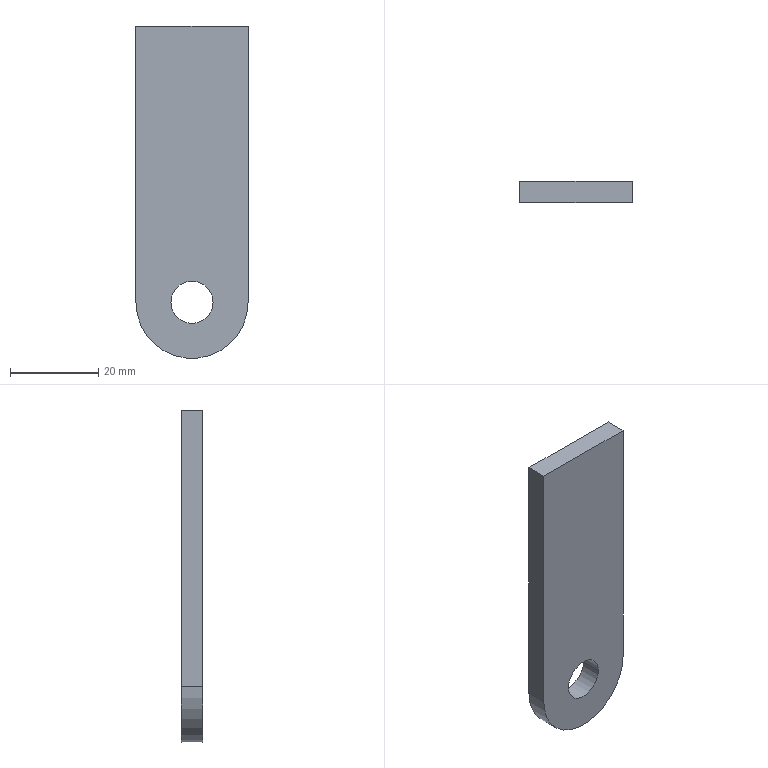Part | NX | features BREP 1 | 1 solid | 8 faces | box 25.4 x 4.763 x 75.311 mm | volume 8439 mm3 | plane 5 | cylinder 3 | commonest cylinder face diameters 9.55 x2 25.4 x1
STEP:
#1=CARTESIAN_POINT('',(12.7,0.,0.));
#2=VERTEX_POINT('',#1);
#3=CARTESIAN_POINT('',(12.7,0.,-62.611));
#4=VERTEX_POINT('',#3);
#5=CARTESIAN_POINT('',(12.7,0.,0.));
#6=DIRECTION('',(0.,0.,-1.));
#7=VECTOR('',#6,1000.);
#8=LINE('',#5,#7);
#9=EDGE_CURVE('',#2,#4,#8,.T.);
#10=ORIENTED_EDGE('',*,*,#9,.T.);
#11=CARTESIAN_POINT('',(-12.7,0.,-62.611));
#12=VERTEX_POINT('',#11);
#13=CARTESIAN_POINT('',(0.,0.,-62.611));
#14=DIRECTION('',(0.,1.,0.));
#15=DIRECTION('',(1.,0.,0.));
#16=AXIS2_PLACEMENT_3D('',#13,#14,#15);
#17=CIRCLE('',#16,12.7);
#18=EDGE_CURVE('',#4,#12,#17,.T.);
#19=ORIENTED_EDGE('',*,*,#18,.T.);
#20=CARTESIAN_POINT('',(-12.7,0.,0.));
#21=VERTEX_POINT('',#20);
#22=CARTESIAN_POINT('',(-12.7,0.,-62.611));
#23=DIRECTION('',(0.,0.,1.));
#24=VECTOR('',#23,1000.);
#25=LINE('',#22,#24);
#26=EDGE_CURVE('',#12,#21,#25,.T.);
#27=ORIENTED_EDGE('',*,*,#26,.T.);
#28=CARTESIAN_POINT('',(-12.7,0.,0.));
#29=DIRECTION('',(1.,0.,0.));
#30=VECTOR('',#29,1000.);
#31=LINE('',#28,#30);
#32=EDGE_CURVE('',#21,#2,#31,.T.);
#33=ORIENTED_EDGE('',*,*,#32,.T.);
#34=EDGE_LOOP('',(#10,#19,#27,#33));
#35=FACE_BOUND('',#34,.T.);
#36=CARTESIAN_POINT('',(4.775,0.,-62.611));
#37=VERTEX_POINT('',#36);
#38=CARTESIAN_POINT('',(-4.775,0.,-62.611));
#39=VERTEX_POINT('',#38);
#40=CARTESIAN_POINT('',(0.,0.,-62.611));
#41=DIRECTION('',(0.,1.,0.));
#42=DIRECTION('',(1.,0.,0.));
#43=AXIS2_PLACEMENT_3D('',#40,#41,#42);
#44=CIRCLE('',#43,4.775);
#45=EDGE_CURVE('',#37,#39,#44,.T.);
#46=ORIENTED_EDGE('',*,*,#45,.F.);
#47=CARTESIAN_POINT('',(0.,0.,-62.611));
#48=DIRECTION('',(0.,1.,0.));
#49=DIRECTION('',(-1.,0.,0.));
#50=AXIS2_PLACEMENT_3D('',#47,#48,#49);
#51=CIRCLE('',#50,4.775);
#52=EDGE_CURVE('',#39,#37,#51,.T.);
#53=ORIENTED_EDGE('',*,*,#52,.F.);
#54=EDGE_LOOP('',(#46,#53));
#55=FACE_BOUND('',#54,.T.);
#56=CARTESIAN_POINT('',(0.,0.,0.));
#57=DIRECTION('',(0.,1.,0.));
#58=DIRECTION('',(1.,0.,0.));
#59=AXIS2_PLACEMENT_3D('',#56,#57,#58);
#60=PLANE('',#59);
#61=ADVANCED_FACE('',(#35,#55),#60,.T.);
#62=CARTESIAN_POINT('',(-12.7,-4.763,0.));
#63=VERTEX_POINT('',#62);
#64=CARTESIAN_POINT('',(-12.7,0.,0.));
#65=DIRECTION('',(0.,-1.,0.));
#66=VECTOR('',#65,1000.);
#67=LINE('',#64,#66);
#68=EDGE_CURVE('',#21,#63,#67,.T.);
#69=ORIENTED_EDGE('',*,*,#68,.T.);
#70=CARTESIAN_POINT('',(12.7,-4.763,0.));
#71=VERTEX_POINT('',#70);
#72=CARTESIAN_POINT('',(-12.7,-4.763,0.));
#73=DIRECTION('',(1.,0.,0.));
#74=VECTOR('',#73,1000.);
#75=LINE('',#72,#74);
#76=EDGE_CURVE('',#63,#71,#75,.T.);
#77=ORIENTED_EDGE('',*,*,#76,.T.);
#78=CARTESIAN_POINT('',(12.7,0.,0.));
#79=DIRECTION('',(0.,-1.,0.));
#80=VECTOR('',#79,1000.);
#81=LINE('',#78,#80);
#82=EDGE_CURVE('',#2,#71,#81,.T.);
#83=ORIENTED_EDGE('',*,*,#82,.F.);
#84=ORIENTED_EDGE('',*,*,#32,.F.);
#85=EDGE_LOOP('',(#69,#77,#83,#84));
#86=FACE_BOUND('',#85,.T.);
#87=CARTESIAN_POINT('',(0.,-2.381,0.));
#88=DIRECTION('',(0.,0.,1.));
#89=DIRECTION('',(1.,0.,0.));
#90=AXIS2_PLACEMENT_3D('',#87,#88,#89);
#91=PLANE('',#90);
#92=ADVANCED_FACE('',(#86),#91,.T.);
#93=ORIENTED_EDGE('',*,*,#82,.T.);
#94=CARTESIAN_POINT('',(12.7,-4.763,-62.611));
#95=VERTEX_POINT('',#94);
#96=CARTESIAN_POINT('',(12.7,-4.763,0.));
#97=DIRECTION('',(0.,0.,-1.));
#98=VECTOR('',#97,1000.);
#99=LINE('',#96,#98);
#100=EDGE_CURVE('',#71,#95,#99,.T.);
#101=ORIENTED_EDGE('',*,*,#100,.T.);
#102=CARTESIAN_POINT('',(12.7,0.,-62.611));
#103=DIRECTION('',(0.,-1.,0.));
#104=VECTOR('',#103,1000.);
#105=LINE('',#102,#104);
#106=EDGE_CURVE('',#4,#95,#105,.T.);
#107=ORIENTED_EDGE('',*,*,#106,.F.);
#108=ORIENTED_EDGE('',*,*,#9,.F.);
#109=EDGE_LOOP('',(#93,#101,#107,#108));
#110=FACE_BOUND('',#109,.T.);
#111=CARTESIAN_POINT('',(12.7,-2.381,-31.305));
#112=DIRECTION('',(1.,0.,0.));
#113=DIRECTION('',(0.,1.,0.));
#114=AXIS2_PLACEMENT_3D('',#111,#112,#113);
#115=PLANE('',#114);
#116=ADVANCED_FACE('',(#110),#115,.T.);
#117=ORIENTED_EDGE('',*,*,#106,.T.);
#118=CARTESIAN_POINT('',(-12.7,-4.763,-62.611));
#119=VERTEX_POINT('',#118);
#120=CARTESIAN_POINT('',(0.,-4.763,-62.611));
#121=DIRECTION('',(0.,1.,0.));
#122=DIRECTION('',(1.,0.,0.));
#123=AXIS2_PLACEMENT_3D('',#120,#121,#122);
#124=CIRCLE('',#123,12.7);
#125=EDGE_CURVE('',#95,#119,#124,.T.);
#126=ORIENTED_EDGE('',*,*,#125,.T.);
#127=CARTESIAN_POINT('',(-12.7,0.,-62.611));
#128=DIRECTION('',(0.,-1.,0.));
#129=VECTOR('',#128,1000.);
#130=LINE('',#127,#129);
#131=EDGE_CURVE('',#12,#119,#130,.T.);
#132=ORIENTED_EDGE('',*,*,#131,.F.);
#133=ORIENTED_EDGE('',*,*,#18,.F.);
#134=EDGE_LOOP('',(#117,#126,#132,#133));
#135=FACE_BOUND('',#134,.T.);
#136=CARTESIAN_POINT('',(0.,-2.381,-62.611));
#137=DIRECTION('',(0.,1.,0.));
#138=DIRECTION('',(1.,0.,0.));
#139=AXIS2_PLACEMENT_3D('',#136,#137,#138);
#140=CYLINDRICAL_SURFACE('',#139,12.7);
#141=ADVANCED_FACE('',(#135),#140,.T.);
#142=ORIENTED_EDGE('',*,*,#131,.T.);
#143=CARTESIAN_POINT('',(-12.7,-4.763,-62.611));
#144=DIRECTION('',(0.,0.,1.));
#145=VECTOR('',#144,1000.);
#146=LINE('',#143,#145);
#147=EDGE_CURVE('',#119,#63,#146,.T.);
#148=ORIENTED_EDGE('',*,*,#147,.T.);
#149=ORIENTED_EDGE('',*,*,#68,.F.);
#150=ORIENTED_EDGE('',*,*,#26,.F.);
#151=EDGE_LOOP('',(#142,#148,#149,#150));
#152=FACE_BOUND('',#151,.T.);
#153=CARTESIAN_POINT('',(-12.7,-2.381,-31.305));
#154=DIRECTION('',(-1.,0.,0.));
#155=DIRECTION('',(0.,0.,1.));
#156=AXIS2_PLACEMENT_3D('',#153,#154,#155);
#157=PLANE('',#156);
#158=ADVANCED_FACE('',(#152),#157,.T.);
#159=ORIENTED_EDGE('',*,*,#147,.F.);
#160=ORIENTED_EDGE('',*,*,#125,.F.);
#161=ORIENTED_EDGE('',*,*,#100,.F.);
#162=ORIENTED_EDGE('',*,*,#76,.F.);
#163=EDGE_LOOP('',(#159,#160,#161,#162));
#164=FACE_BOUND('',#163,.T.);
#165=CARTESIAN_POINT('',(4.775,-4.763,-62.611));
#166=VERTEX_POINT('',#165);
#167=CARTESIAN_POINT('',(-4.775,-4.763,-62.611));
#168=VERTEX_POINT('',#167);
#169=CARTESIAN_POINT('',(0.,-4.763,-62.611));
#170=DIRECTION('',(0.,1.,0.));
#171=DIRECTION('',(1.,0.,0.));
#172=AXIS2_PLACEMENT_3D('',#169,#170,#171);
#173=CIRCLE('',#172,4.775);
#174=EDGE_CURVE('',#166,#168,#173,.T.);
#175=ORIENTED_EDGE('',*,*,#174,.T.);
#176=CARTESIAN_POINT('',(0.,-4.763,-62.611));
#177=DIRECTION('',(0.,1.,0.));
#178=DIRECTION('',(-1.,0.,0.));
#179=AXIS2_PLACEMENT_3D('',#176,#177,#178);
#180=CIRCLE('',#179,4.775);
#181=EDGE_CURVE('',#168,#166,#180,.T.);
#182=ORIENTED_EDGE('',*,*,#181,.T.);
#183=EDGE_LOOP('',(#175,#182));
#184=FACE_BOUND('',#183,.T.);
#185=CARTESIAN_POINT('',(0.,-4.763,0.));
#186=DIRECTION('',(0.,1.,0.));
#187=DIRECTION('',(1.,0.,0.));
#188=AXIS2_PLACEMENT_3D('',#185,#186,#187);
#189=PLANE('',#188);
#190=ADVANCED_FACE('',(#164,#184),#189,.F.);
#191=CARTESIAN_POINT('',(4.775,0.,-62.611));
#192=DIRECTION('',(0.,-1.,0.));
#193=VECTOR('',#192,1000.);
#194=LINE('',#191,#193);
#195=EDGE_CURVE('',#166,#37,#194,.F.);
#196=ORIENTED_EDGE('',*,*,#195,.F.);
#197=ORIENTED_EDGE('',*,*,#181,.F.);
#198=CARTESIAN_POINT('',(-4.775,0.,-62.611));
#199=DIRECTION('',(0.,-1.,0.));
#200=VECTOR('',#199,1000.);
#201=LINE('',#198,#200);
#202=EDGE_CURVE('',#168,#39,#201,.F.);
#203=ORIENTED_EDGE('',*,*,#202,.T.);
#204=ORIENTED_EDGE('',*,*,#52,.T.);
#205=EDGE_LOOP('',(#196,#197,#203,#204));
#206=FACE_BOUND('',#205,.T.);
#207=CARTESIAN_POINT('',(0.,-2.381,-62.611));
#208=DIRECTION('',(0.,1.,0.));
#209=DIRECTION('',(-1.,0.,0.));
#210=AXIS2_PLACEMENT_3D('',#207,#208,#209);
#211=CYLINDRICAL_SURFACE('',#210,4.775);
#212=ADVANCED_FACE('',(#206),#211,.F.);
#213=ORIENTED_EDGE('',*,*,#202,.F.);
#214=ORIENTED_EDGE('',*,*,#174,.F.);
#215=ORIENTED_EDGE('',*,*,#195,.T.);
#216=ORIENTED_EDGE('',*,*,#45,.T.);
#217=EDGE_LOOP('',(#213,#214,#215,#216));
#218=FACE_BOUND('',#217,.T.);
#219=CARTESIAN_POINT('',(0.,-2.381,-62.611));
#220=DIRECTION('',(0.,1.,0.));
#221=DIRECTION('',(1.,0.,0.));
#222=AXIS2_PLACEMENT_3D('',#219,#220,#221);
#223=CYLINDRICAL_SURFACE('',#222,4.775);
#224=ADVANCED_FACE('',(#218),#223,.F.);
#225=CLOSED_SHELL('',(#61,#92,#116,#141,#158,#190,#212,#224));
#226=MANIFOLD_SOLID_BREP('',#225);
#227=(LENGTH_UNIT()NAMED_UNIT(*)SI_UNIT(.MILLI.,.METRE.));
#228=UNCERTAINTY_MEASURE_WITH_UNIT(LENGTH_MEASURE(0.00001),#227,'','');
#229=(NAMED_UNIT(*)PLANE_ANGLE_UNIT()SI_UNIT($,.RADIAN.));
#230=(NAMED_UNIT(*)SI_UNIT($,.STERADIAN.)SOLID_ANGLE_UNIT());
#231=(GEOMETRIC_REPRESENTATION_CONTEXT(3)GLOBAL_UNCERTAINTY_ASSIGNED_CONTEXT((#228))GLOBAL_UNIT_ASSIGNED_CONTEXT((#227,#229,#230))REPRESENTATION_CONTEXT('',''));
#232=ADVANCED_BREP_SHAPE_REPRESENTATION('',(#226),#231);